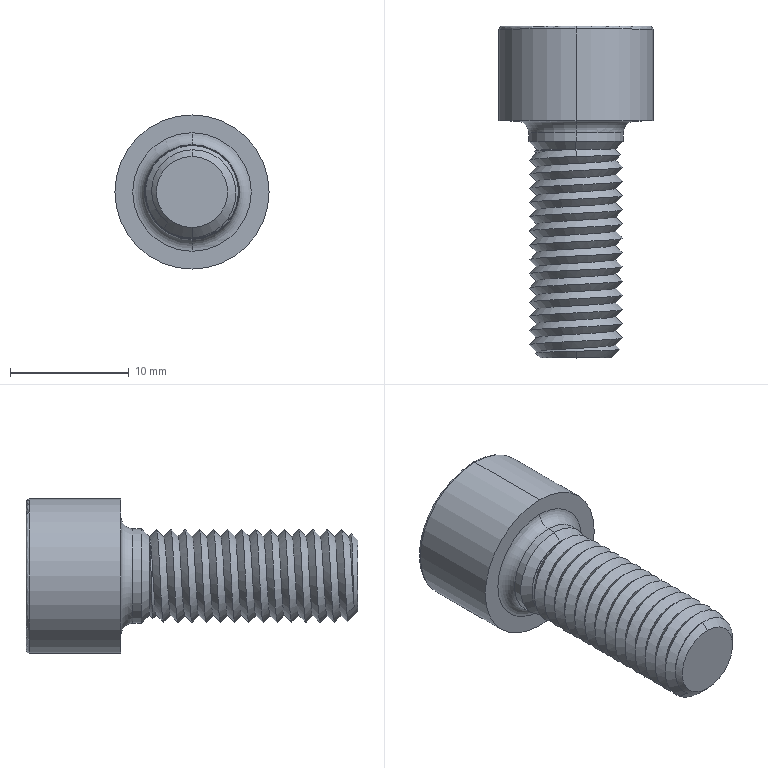Part | STEP file | Parafuso M8 - 20mm | 1 solid | 36 faces | box 13 x 28 x 13 mm | volume 1700 mm3 | plane 16 | cone 8 | torus 6 | cylinder 4 | spline 2 | commonest cylinder face diameters 8 x2 13 x2